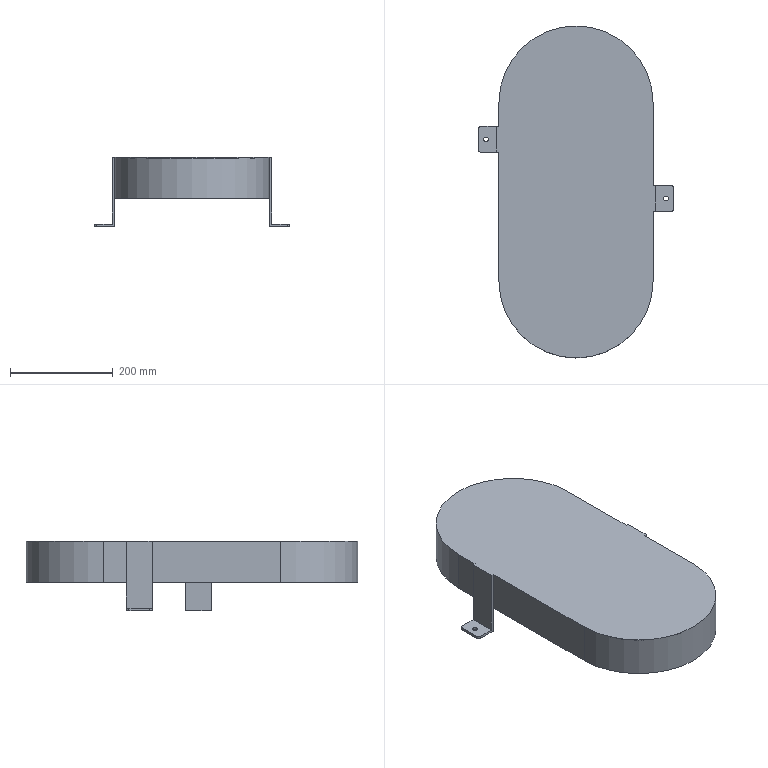Part | STEP file | Part 1 | 1 solid | 37 faces | box 380 x 645.065 x 135 mm | volume 686374 mm3 | plane 23 | cylinder 14 | commonest cylinder face diameters 9 x4 10 x4 296 x3 300 x3